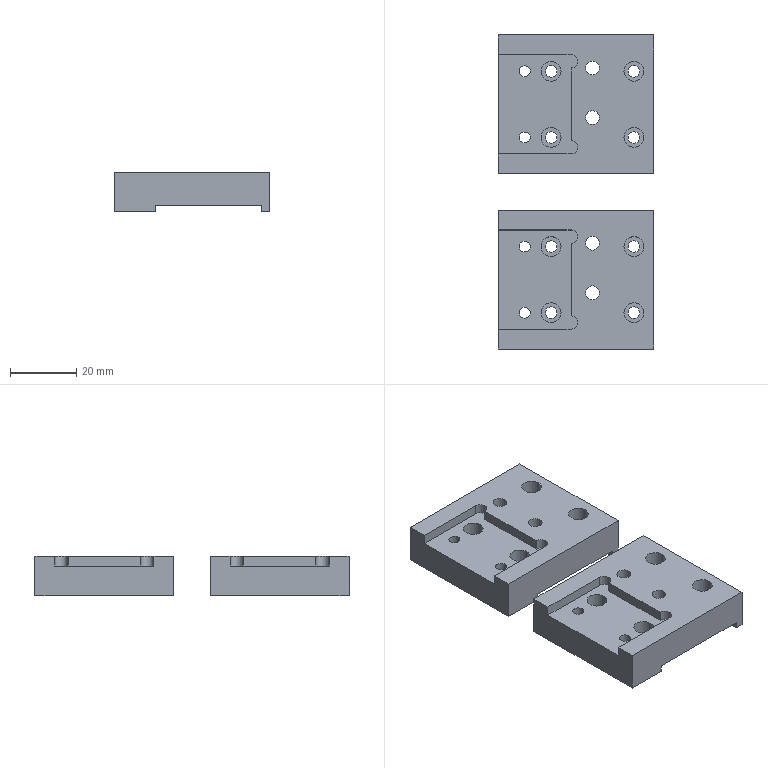Part | 2 solids | 88 faces | box 47 x 95 x 12 mm | volume 35478 mm3 | cylinder 52 | plane 36 | commonest cylinder face diameters 3.5 x16 6 x16 3.3 x8 4.2 x8 4 x4